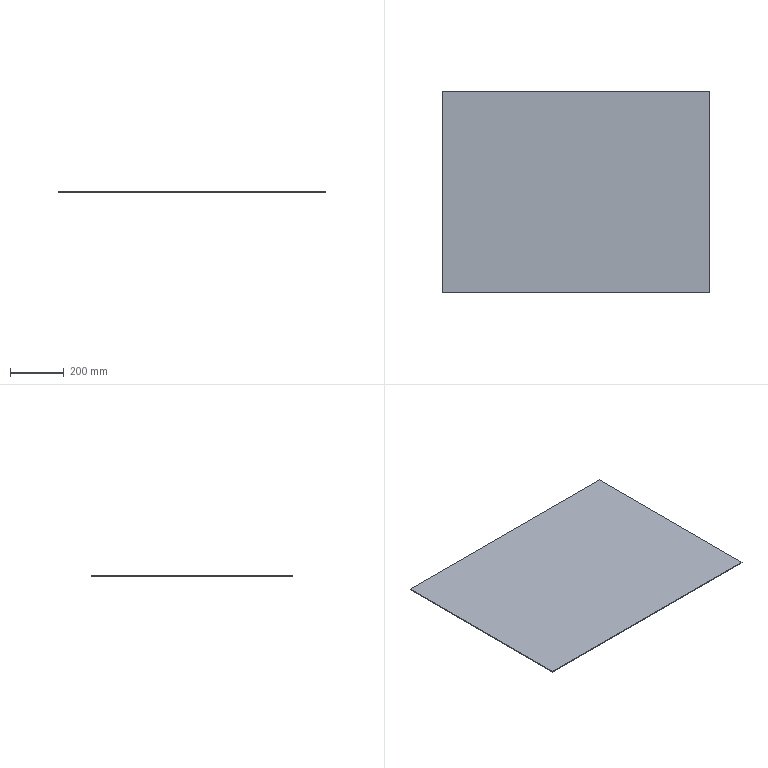Part | SolidWorks | features Extrusion 1 | 1 solid | 6 faces | box 1000 x 755 x 3 mm | volume 2265000 mm3 | plane 6
STEP:
#1=CARTESIAN_POINT('',(0.,755.,0.));
#2=VERTEX_POINT('',#1);
#3=CARTESIAN_POINT('',(0.,0.,0.));
#4=VERTEX_POINT('',#3);
#5=CARTESIAN_POINT('',(0.,0.,0.));
#6=DIRECTION('',(0.,-1.,0.));
#7=VECTOR('',#6,1000.);
#8=LINE('',#5,#7);
#9=EDGE_CURVE('',#2,#4,#8,.T.);
#10=ORIENTED_EDGE('',*,*,#9,.T.);
#11=CARTESIAN_POINT('',(0.,0.,3.));
#12=VERTEX_POINT('',#11);
#13=CARTESIAN_POINT('',(0.,0.,3.));
#14=DIRECTION('',(0.,0.,-1.));
#15=VECTOR('',#14,1000.);
#16=LINE('',#13,#15);
#17=EDGE_CURVE('',#12,#4,#16,.T.);
#18=ORIENTED_EDGE('',*,*,#17,.F.);
#19=CARTESIAN_POINT('',(0.,755.,3.));
#20=VERTEX_POINT('',#19);
#21=CARTESIAN_POINT('',(0.,0.,3.));
#22=DIRECTION('',(0.,-1.,0.));
#23=VECTOR('',#22,1000.);
#24=LINE('',#21,#23);
#25=EDGE_CURVE('',#20,#12,#24,.T.);
#26=ORIENTED_EDGE('',*,*,#25,.F.);
#27=CARTESIAN_POINT('',(0.,755.,3.));
#28=DIRECTION('',(0.,0.,-1.));
#29=VECTOR('',#28,1000.);
#30=LINE('',#27,#29);
#31=EDGE_CURVE('',#20,#2,#30,.T.);
#32=ORIENTED_EDGE('',*,*,#31,.T.);
#33=EDGE_LOOP('',(#10,#18,#26,#32));
#34=FACE_OUTER_BOUND('',#33,.T.);
#35=CARTESIAN_POINT('',(0.,0.,3.));
#36=DIRECTION('',(1.,0.,0.));
#37=DIRECTION('',(0.,0.,-1.));
#38=AXIS2_PLACEMENT_3D('',#35,#36,#37);
#39=PLANE('',#38);
#40=ADVANCED_FACE('',(#34),#39,.F.);
#41=CARTESIAN_POINT('',(1000.,0.,0.));
#42=VERTEX_POINT('',#41);
#43=CARTESIAN_POINT('',(0.,0.,0.));
#44=DIRECTION('',(1.,0.,0.));
#45=VECTOR('',#44,1000.);
#46=LINE('',#43,#45);
#47=EDGE_CURVE('',#4,#42,#46,.T.);
#48=ORIENTED_EDGE('',*,*,#47,.T.);
#49=CARTESIAN_POINT('',(1000.,0.,3.));
#50=VERTEX_POINT('',#49);
#51=CARTESIAN_POINT('',(1000.,0.,3.));
#52=DIRECTION('',(0.,0.,-1.));
#53=VECTOR('',#52,1000.);
#54=LINE('',#51,#53);
#55=EDGE_CURVE('',#50,#42,#54,.T.);
#56=ORIENTED_EDGE('',*,*,#55,.F.);
#57=CARTESIAN_POINT('',(0.,0.,3.));
#58=DIRECTION('',(1.,0.,0.));
#59=VECTOR('',#58,1000.);
#60=LINE('',#57,#59);
#61=EDGE_CURVE('',#12,#50,#60,.T.);
#62=ORIENTED_EDGE('',*,*,#61,.F.);
#63=ORIENTED_EDGE('',*,*,#17,.T.);
#64=EDGE_LOOP('',(#48,#56,#62,#63));
#65=FACE_OUTER_BOUND('',#64,.T.);
#66=CARTESIAN_POINT('',(0.,0.,3.));
#67=DIRECTION('',(0.,1.,0.));
#68=DIRECTION('',(0.,0.,1.));
#69=AXIS2_PLACEMENT_3D('',#66,#67,#68);
#70=PLANE('',#69);
#71=ADVANCED_FACE('',(#65),#70,.F.);
#72=CARTESIAN_POINT('',(1000.,755.,0.));
#73=VERTEX_POINT('',#72);
#74=CARTESIAN_POINT('',(1000.,0.,0.));
#75=DIRECTION('',(0.,1.,0.));
#76=VECTOR('',#75,1000.);
#77=LINE('',#74,#76);
#78=EDGE_CURVE('',#42,#73,#77,.T.);
#79=ORIENTED_EDGE('',*,*,#78,.T.);
#80=CARTESIAN_POINT('',(1000.,755.,3.));
#81=VERTEX_POINT('',#80);
#82=CARTESIAN_POINT('',(1000.,755.,3.));
#83=DIRECTION('',(0.,0.,-1.));
#84=VECTOR('',#83,1000.);
#85=LINE('',#82,#84);
#86=EDGE_CURVE('',#81,#73,#85,.T.);
#87=ORIENTED_EDGE('',*,*,#86,.F.);
#88=CARTESIAN_POINT('',(1000.,0.,3.));
#89=DIRECTION('',(0.,1.,0.));
#90=VECTOR('',#89,1000.);
#91=LINE('',#88,#90);
#92=EDGE_CURVE('',#50,#81,#91,.T.);
#93=ORIENTED_EDGE('',*,*,#92,.F.);
#94=ORIENTED_EDGE('',*,*,#55,.T.);
#95=EDGE_LOOP('',(#79,#87,#93,#94));
#96=FACE_OUTER_BOUND('',#95,.T.);
#97=CARTESIAN_POINT('',(1000.,0.,3.));
#98=DIRECTION('',(-1.,0.,0.));
#99=DIRECTION('',(0.,0.,1.));
#100=AXIS2_PLACEMENT_3D('',#97,#98,#99);
#101=PLANE('',#100);
#102=ADVANCED_FACE('',(#96),#101,.F.);
#103=CARTESIAN_POINT('',(0.,755.,0.));
#104=DIRECTION('',(-1.,0.,0.));
#105=VECTOR('',#104,1000.);
#106=LINE('',#103,#105);
#107=EDGE_CURVE('',#73,#2,#106,.T.);
#108=ORIENTED_EDGE('',*,*,#107,.T.);
#109=ORIENTED_EDGE('',*,*,#31,.F.);
#110=CARTESIAN_POINT('',(0.,755.,3.));
#111=DIRECTION('',(-1.,0.,0.));
#112=VECTOR('',#111,1000.);
#113=LINE('',#110,#112);
#114=EDGE_CURVE('',#81,#20,#113,.T.);
#115=ORIENTED_EDGE('',*,*,#114,.F.);
#116=ORIENTED_EDGE('',*,*,#86,.T.);
#117=EDGE_LOOP('',(#108,#109,#115,#116));
#118=FACE_OUTER_BOUND('',#117,.T.);
#119=CARTESIAN_POINT('',(0.,755.,3.));
#120=DIRECTION('',(0.,-1.,0.));
#121=DIRECTION('',(0.,0.,-1.));
#122=AXIS2_PLACEMENT_3D('',#119,#120,#121);
#123=PLANE('',#122);
#124=ADVANCED_FACE('',(#118),#123,.F.);
#125=ORIENTED_EDGE('',*,*,#25,.T.);
#126=ORIENTED_EDGE('',*,*,#61,.T.);
#127=ORIENTED_EDGE('',*,*,#92,.T.);
#128=ORIENTED_EDGE('',*,*,#114,.T.);
#129=EDGE_LOOP('',(#125,#126,#127,#128));
#130=FACE_OUTER_BOUND('',#129,.T.);
#131=CARTESIAN_POINT('',(0.,0.,3.));
#132=DIRECTION('',(0.,0.,-1.));
#133=DIRECTION('',(-1.,0.,0.));
#134=AXIS2_PLACEMENT_3D('',#131,#132,#133);
#135=PLANE('',#134);
#136=ADVANCED_FACE('',(#130),#135,.F.);
#137=ORIENTED_EDGE('',*,*,#9,.F.);
#138=ORIENTED_EDGE('',*,*,#107,.F.);
#139=ORIENTED_EDGE('',*,*,#78,.F.);
#140=ORIENTED_EDGE('',*,*,#47,.F.);
#141=EDGE_LOOP('',(#137,#138,#139,#140));
#142=FACE_OUTER_BOUND('',#141,.T.);
#143=CARTESIAN_POINT('',(0.,0.,0.));
#144=DIRECTION('',(0.,0.,-1.));
#145=DIRECTION('',(-1.,0.,0.));
#146=AXIS2_PLACEMENT_3D('',#143,#144,#145);
#147=PLANE('',#146);
#148=ADVANCED_FACE('',(#142),#147,.T.);
#149=CLOSED_SHELL('',(#40,#71,#102,#124,#136,#148));
#150=MANIFOLD_SOLID_BREP('',#149);
#151=CARTESIAN_POINT('',(0.,0.,0.));
#152=DIRECTION('',(0.,0.,1.));
#153=DIRECTION('',(1.,0.,0.));
#154=AXIS2_PLACEMENT_3D('',#151,#152,#153);
#155=(LENGTH_UNIT()NAMED_UNIT(*)SI_UNIT(.MILLI.,.METRE.));
#156=UNCERTAINTY_MEASURE_WITH_UNIT(LENGTH_MEASURE(0.00001),#155,'','');
#157=(NAMED_UNIT(*)PLANE_ANGLE_UNIT()SI_UNIT($,.RADIAN.));
#158=(NAMED_UNIT(*)SI_UNIT($,.STERADIAN.)SOLID_ANGLE_UNIT());
#159=(GEOMETRIC_REPRESENTATION_CONTEXT(3)GLOBAL_UNCERTAINTY_ASSIGNED_CONTEXT((#156))GLOBAL_UNIT_ASSIGNED_CONTEXT((#155,#157,#158))REPRESENTATION_CONTEXT('',''));
#160=ADVANCED_BREP_SHAPE_REPRESENTATION('',(#150,#154),#159);